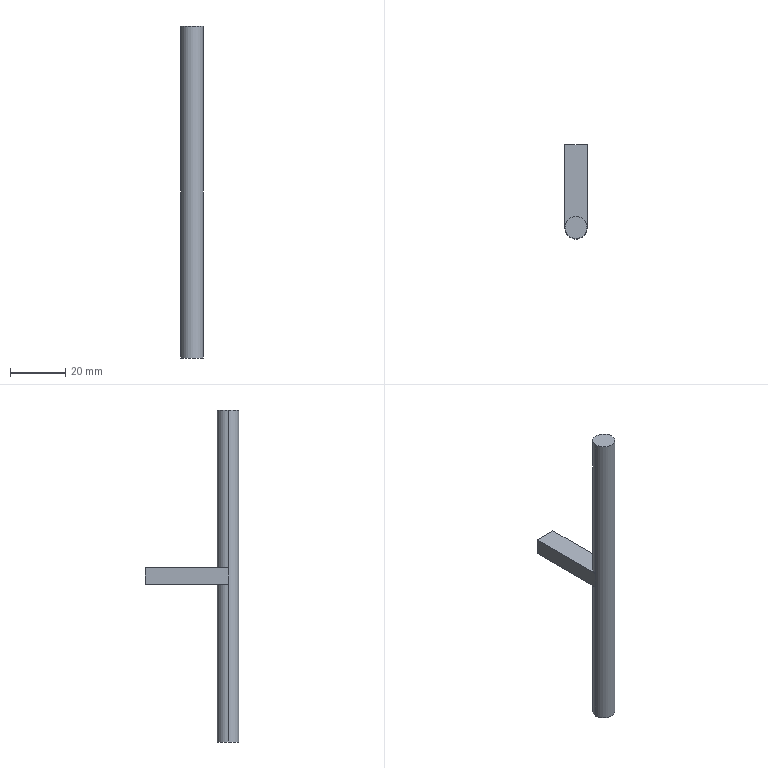Part | SolidWorks | features Extrusion 1, ICE 1 | 1 solid | 10 faces | box 8 x 34 x 120 mm | volume 7321 mm3 | plane 7 | cylinder 3 | commonest cylinder face diameters 8 x3
STEP:
#1=CARTESIAN_POINT('',(4.,0.,120.));
#2=VERTEX_POINT('',#1);
#3=CARTESIAN_POINT('',(-4.,0.,120.));
#4=VERTEX_POINT('',#3);
#5=CARTESIAN_POINT('',(0.,0.,120.));
#6=DIRECTION('',(0.,0.,1.));
#7=DIRECTION('',(1.,0.,0.));
#8=AXIS2_PLACEMENT_3D('',#5,#6,#7);
#9=CIRCLE('',#8,4.);
#10=EDGE_CURVE('',#2,#4,#9,.T.);
#11=ORIENTED_EDGE('',*,*,#10,.F.);
#12=CARTESIAN_POINT('',(4.,0.,63.));
#13=VERTEX_POINT('',#12);
#14=CARTESIAN_POINT('',(4.,0.,120.));
#15=DIRECTION('',(0.,0.,-1.));
#16=VECTOR('',#15,1000.);
#17=LINE('',#14,#16);
#18=EDGE_CURVE('',#2,#13,#17,.T.);
#19=ORIENTED_EDGE('',*,*,#18,.T.);
#20=CARTESIAN_POINT('',(-4.,0.,63.));
#21=VERTEX_POINT('',#20);
#22=CARTESIAN_POINT('',(0.,0.,63.));
#23=DIRECTION('',(0.,0.,-1.));
#24=DIRECTION('',(-1.,0.,0.));
#25=AXIS2_PLACEMENT_3D('',#22,#23,#24);
#26=CIRCLE('',#25,4.);
#27=EDGE_CURVE('',#21,#13,#26,.T.);
#28=ORIENTED_EDGE('',*,*,#27,.F.);
#29=CARTESIAN_POINT('',(-4.,0.,120.));
#30=DIRECTION('',(0.,0.,-1.));
#31=VECTOR('',#30,1000.);
#32=LINE('',#29,#31);
#33=EDGE_CURVE('',#4,#21,#32,.T.);
#34=ORIENTED_EDGE('',*,*,#33,.F.);
#35=EDGE_LOOP('',(#11,#19,#28,#34));
#36=FACE_OUTER_BOUND('',#35,.T.);
#37=CARTESIAN_POINT('',(0.,0.,120.));
#38=DIRECTION('',(0.,0.,-1.));
#39=DIRECTION('',(-1.,0.,0.));
#40=AXIS2_PLACEMENT_3D('',#37,#38,#39);
#41=CYLINDRICAL_SURFACE('',#40,4.);
#42=ADVANCED_FACE('',(#36),#41,.T.);
#43=CARTESIAN_POINT('',(4.,0.,57.));
#44=VERTEX_POINT('',#43);
#45=CARTESIAN_POINT('',(-4.,0.,57.));
#46=VERTEX_POINT('',#45);
#47=CARTESIAN_POINT('',(0.,0.,57.));
#48=DIRECTION('',(0.,0.,1.));
#49=DIRECTION('',(1.,0.,0.));
#50=AXIS2_PLACEMENT_3D('',#47,#48,#49);
#51=CIRCLE('',#50,4.);
#52=EDGE_CURVE('',#44,#46,#51,.T.);
#53=ORIENTED_EDGE('',*,*,#52,.F.);
#54=CARTESIAN_POINT('',(4.,0.,0.));
#55=VERTEX_POINT('',#54);
#56=CARTESIAN_POINT('',(4.,0.,120.));
#57=DIRECTION('',(0.,0.,-1.));
#58=VECTOR('',#57,1000.);
#59=LINE('',#56,#58);
#60=EDGE_CURVE('',#44,#55,#59,.T.);
#61=ORIENTED_EDGE('',*,*,#60,.T.);
#62=CARTESIAN_POINT('',(-4.,0.,0.));
#63=VERTEX_POINT('',#62);
#64=CARTESIAN_POINT('',(0.,0.,0.));
#65=DIRECTION('',(0.,0.,1.));
#66=DIRECTION('',(1.,0.,0.));
#67=AXIS2_PLACEMENT_3D('',#64,#65,#66);
#68=CIRCLE('',#67,4.);
#69=EDGE_CURVE('',#55,#63,#68,.T.);
#70=ORIENTED_EDGE('',*,*,#69,.T.);
#71=CARTESIAN_POINT('',(-4.,0.,120.));
#72=DIRECTION('',(0.,0.,-1.));
#73=VECTOR('',#72,1000.);
#74=LINE('',#71,#73);
#75=EDGE_CURVE('',#46,#63,#74,.T.);
#76=ORIENTED_EDGE('',*,*,#75,.F.);
#77=EDGE_LOOP('',(#53,#61,#70,#76));
#78=FACE_OUTER_BOUND('',#77,.T.);
#79=CARTESIAN_POINT('',(0.,0.,120.));
#80=DIRECTION('',(0.,0.,-1.));
#81=DIRECTION('',(-1.,0.,0.));
#82=AXIS2_PLACEMENT_3D('',#79,#80,#81);
#83=CYLINDRICAL_SURFACE('',#82,4.);
#84=ADVANCED_FACE('',(#78),#83,.T.);
#85=ORIENTED_EDGE('',*,*,#18,.F.);
#86=CARTESIAN_POINT('',(0.,0.,120.));
#87=DIRECTION('',(0.,0.,1.));
#88=DIRECTION('',(1.,0.,0.));
#89=AXIS2_PLACEMENT_3D('',#86,#87,#88);
#90=CIRCLE('',#89,4.);
#91=EDGE_CURVE('',#4,#2,#90,.T.);
#92=ORIENTED_EDGE('',*,*,#91,.F.);
#93=ORIENTED_EDGE('',*,*,#33,.T.);
#94=CARTESIAN_POINT('',(-4.,0.,57.));
#95=DIRECTION('',(0.,0.,1.));
#96=VECTOR('',#95,1000.);
#97=LINE('',#94,#96);
#98=EDGE_CURVE('',#46,#21,#97,.T.);
#99=ORIENTED_EDGE('',*,*,#98,.F.);
#100=ORIENTED_EDGE('',*,*,#75,.T.);
#101=CARTESIAN_POINT('',(0.,0.,0.));
#102=DIRECTION('',(0.,0.,1.));
#103=DIRECTION('',(1.,0.,0.));
#104=AXIS2_PLACEMENT_3D('',#101,#102,#103);
#105=CIRCLE('',#104,4.);
#106=EDGE_CURVE('',#63,#55,#105,.T.);
#107=ORIENTED_EDGE('',*,*,#106,.T.);
#108=ORIENTED_EDGE('',*,*,#60,.F.);
#109=CARTESIAN_POINT('',(4.,0.,57.));
#110=DIRECTION('',(0.,0.,-1.));
#111=VECTOR('',#110,1000.);
#112=LINE('',#109,#111);
#113=EDGE_CURVE('',#13,#44,#112,.T.);
#114=ORIENTED_EDGE('',*,*,#113,.F.);
#115=EDGE_LOOP('',(#85,#92,#93,#99,#100,#107,#108,#114));
#116=FACE_OUTER_BOUND('',#115,.T.);
#117=CARTESIAN_POINT('',(0.,0.,120.));
#118=DIRECTION('',(0.,0.,-1.));
#119=DIRECTION('',(-1.,0.,0.));
#120=AXIS2_PLACEMENT_3D('',#117,#118,#119);
#121=CYLINDRICAL_SURFACE('',#120,4.);
#122=ADVANCED_FACE('',(#116),#121,.T.);
#123=ORIENTED_EDGE('',*,*,#91,.T.);
#124=ORIENTED_EDGE('',*,*,#10,.T.);
#125=EDGE_LOOP('',(#123,#124));
#126=FACE_OUTER_BOUND('',#125,.T.);
#127=CARTESIAN_POINT('',(0.,0.,120.));
#128=DIRECTION('',(0.,0.,1.));
#129=DIRECTION('',(1.,0.,0.));
#130=AXIS2_PLACEMENT_3D('',#127,#128,#129);
#131=PLANE('',#130);
#132=ADVANCED_FACE('',(#126),#131,.T.);
#133=ORIENTED_EDGE('',*,*,#106,.F.);
#134=ORIENTED_EDGE('',*,*,#69,.F.);
#135=EDGE_LOOP('',(#133,#134));
#136=FACE_OUTER_BOUND('',#135,.T.);
#137=CARTESIAN_POINT('',(0.,0.,0.));
#138=DIRECTION('',(0.,0.,1.));
#139=DIRECTION('',(1.,0.,0.));
#140=AXIS2_PLACEMENT_3D('',#137,#138,#139);
#141=PLANE('',#140);
#142=ADVANCED_FACE('',(#136),#141,.F.);
#143=ORIENTED_EDGE('',*,*,#113,.T.);
#144=CARTESIAN_POINT('',(4.,30.,57.));
#145=VERTEX_POINT('',#144);
#146=CARTESIAN_POINT('',(4.,30.,57.));
#147=DIRECTION('',(0.,-1.,0.));
#148=VECTOR('',#147,1000.);
#149=LINE('',#146,#148);
#150=EDGE_CURVE('',#145,#44,#149,.T.);
#151=ORIENTED_EDGE('',*,*,#150,.F.);
#152=CARTESIAN_POINT('',(4.,30.,63.));
#153=VERTEX_POINT('',#152);
#154=CARTESIAN_POINT('',(4.,30.,57.));
#155=DIRECTION('',(0.,0.,-1.));
#156=VECTOR('',#155,1000.);
#157=LINE('',#154,#156);
#158=EDGE_CURVE('',#153,#145,#157,.T.);
#159=ORIENTED_EDGE('',*,*,#158,.F.);
#160=CARTESIAN_POINT('',(4.,30.,63.));
#161=DIRECTION('',(0.,-1.,0.));
#162=VECTOR('',#161,1000.);
#163=LINE('',#160,#162);
#164=EDGE_CURVE('',#153,#13,#163,.T.);
#165=ORIENTED_EDGE('',*,*,#164,.T.);
#166=EDGE_LOOP('',(#143,#151,#159,#165));
#167=FACE_OUTER_BOUND('',#166,.T.);
#168=CARTESIAN_POINT('',(4.,30.,57.));
#169=DIRECTION('',(-1.,0.,0.));
#170=DIRECTION('',(0.,0.,1.));
#171=AXIS2_PLACEMENT_3D('',#168,#169,#170);
#172=PLANE('',#171);
#173=ADVANCED_FACE('',(#167),#172,.F.);
#174=ORIENTED_EDGE('',*,*,#150,.T.);
#175=ORIENTED_EDGE('',*,*,#52,.T.);
#176=CARTESIAN_POINT('',(-4.,30.,57.));
#177=VERTEX_POINT('',#176);
#178=CARTESIAN_POINT('',(-4.,30.,57.));
#179=DIRECTION('',(0.,-1.,0.));
#180=VECTOR('',#179,1000.);
#181=LINE('',#178,#180);
#182=EDGE_CURVE('',#177,#46,#181,.T.);
#183=ORIENTED_EDGE('',*,*,#182,.F.);
#184=CARTESIAN_POINT('',(-4.,30.,57.));
#185=DIRECTION('',(-1.,0.,0.));
#186=VECTOR('',#185,1000.);
#187=LINE('',#184,#186);
#188=EDGE_CURVE('',#145,#177,#187,.T.);
#189=ORIENTED_EDGE('',*,*,#188,.F.);
#190=EDGE_LOOP('',(#174,#175,#183,#189));
#191=FACE_OUTER_BOUND('',#190,.T.);
#192=CARTESIAN_POINT('',(-4.,30.,57.));
#193=DIRECTION('',(0.,0.,1.));
#194=DIRECTION('',(1.,0.,0.));
#195=AXIS2_PLACEMENT_3D('',#192,#193,#194);
#196=PLANE('',#195);
#197=ADVANCED_FACE('',(#191),#196,.F.);
#198=ORIENTED_EDGE('',*,*,#98,.T.);
#199=CARTESIAN_POINT('',(-4.,30.,63.));
#200=VERTEX_POINT('',#199);
#201=CARTESIAN_POINT('',(-4.,30.,63.));
#202=DIRECTION('',(0.,-1.,0.));
#203=VECTOR('',#202,1000.);
#204=LINE('',#201,#203);
#205=EDGE_CURVE('',#200,#21,#204,.T.);
#206=ORIENTED_EDGE('',*,*,#205,.F.);
#207=CARTESIAN_POINT('',(-4.,30.,57.));
#208=DIRECTION('',(0.,0.,1.));
#209=VECTOR('',#208,1000.);
#210=LINE('',#207,#209);
#211=EDGE_CURVE('',#177,#200,#210,.T.);
#212=ORIENTED_EDGE('',*,*,#211,.F.);
#213=ORIENTED_EDGE('',*,*,#182,.T.);
#214=EDGE_LOOP('',(#198,#206,#212,#213));
#215=FACE_OUTER_BOUND('',#214,.T.);
#216=CARTESIAN_POINT('',(-4.,30.,57.));
#217=DIRECTION('',(1.,0.,0.));
#218=DIRECTION('',(0.,0.,-1.));
#219=AXIS2_PLACEMENT_3D('',#216,#217,#218);
#220=PLANE('',#219);
#221=ADVANCED_FACE('',(#215),#220,.F.);
#222=ORIENTED_EDGE('',*,*,#205,.T.);
#223=ORIENTED_EDGE('',*,*,#27,.T.);
#224=ORIENTED_EDGE('',*,*,#164,.F.);
#225=CARTESIAN_POINT('',(-4.,30.,63.));
#226=DIRECTION('',(1.,0.,0.));
#227=VECTOR('',#226,1000.);
#228=LINE('',#225,#227);
#229=EDGE_CURVE('',#200,#153,#228,.T.);
#230=ORIENTED_EDGE('',*,*,#229,.F.);
#231=EDGE_LOOP('',(#222,#223,#224,#230));
#232=FACE_OUTER_BOUND('',#231,.T.);
#233=CARTESIAN_POINT('',(-4.,30.,63.));
#234=DIRECTION('',(0.,0.,-1.));
#235=DIRECTION('',(-1.,0.,0.));
#236=AXIS2_PLACEMENT_3D('',#233,#234,#235);
#237=PLANE('',#236);
#238=ADVANCED_FACE('',(#232),#237,.F.);
#239=ORIENTED_EDGE('',*,*,#158,.T.);
#240=ORIENTED_EDGE('',*,*,#188,.T.);
#241=ORIENTED_EDGE('',*,*,#211,.T.);
#242=ORIENTED_EDGE('',*,*,#229,.T.);
#243=EDGE_LOOP('',(#239,#240,#241,#242));
#244=FACE_OUTER_BOUND('',#243,.T.);
#245=CARTESIAN_POINT('',(0.,30.,0.));
#246=DIRECTION('',(0.,1.,0.));
#247=DIRECTION('',(0.,0.,1.));
#248=AXIS2_PLACEMENT_3D('',#245,#246,#247);
#249=PLANE('',#248);
#250=ADVANCED_FACE('',(#244),#249,.T.);
#251=CLOSED_SHELL('',(#42,#84,#122,#132,#142,#173,#197,#221,#238,#250));
#252=MANIFOLD_SOLID_BREP('',#251);
#253=CARTESIAN_POINT('',(0.,0.,0.));
#254=DIRECTION('',(0.,0.,1.));
#255=DIRECTION('',(1.,0.,0.));
#256=AXIS2_PLACEMENT_3D('',#253,#254,#255);
#257=(LENGTH_UNIT()NAMED_UNIT(*)SI_UNIT(.MILLI.,.METRE.));
#258=UNCERTAINTY_MEASURE_WITH_UNIT(LENGTH_MEASURE(0.00001),#257,'','');
#259=(NAMED_UNIT(*)PLANE_ANGLE_UNIT()SI_UNIT($,.RADIAN.));
#260=(NAMED_UNIT(*)SI_UNIT($,.STERADIAN.)SOLID_ANGLE_UNIT());
#261=(GEOMETRIC_REPRESENTATION_CONTEXT(3)GLOBAL_UNCERTAINTY_ASSIGNED_CONTEXT((#258))GLOBAL_UNIT_ASSIGNED_CONTEXT((#257,#259,#260))REPRESENTATION_CONTEXT('',''));
#262=ADVANCED_BREP_SHAPE_REPRESENTATION('',(#252,#256),#261);